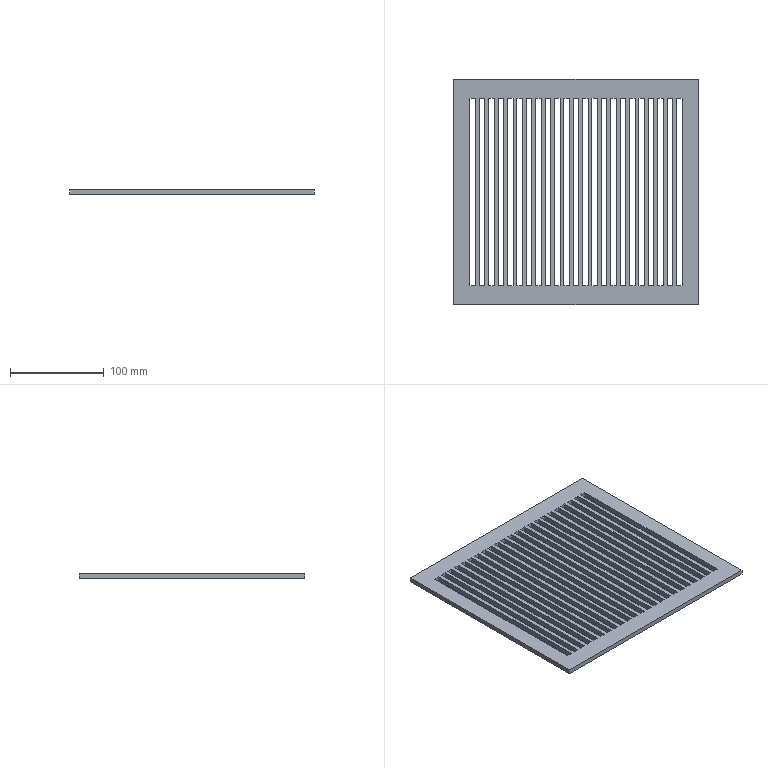Part | SolidWorks | features Extrusion 1, ICE 1, LPattern 1 | 1 solid | 98 faces | box 260 x 240 x 5 mm | volume 174000 mm3 | plane 98